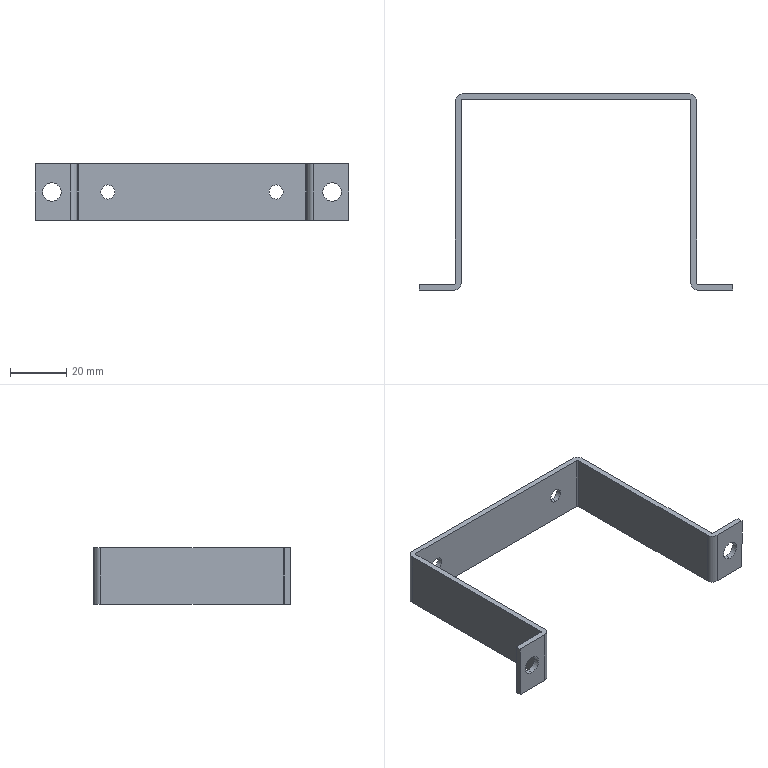Part | STEP file | Support sheet metal | 1 solid | 30 faces | box 112 x 70 x 20 mm | volume 9602 mm3 | cylinder 16 | plane 14 | commonest cylinder face diameters 5 x8 1 x4 6.6 x4
STEP:
#1=CARTESIAN_POINT('',(30.,-2.,-2.5));
#2=VERTEX_POINT('',#1);
#3=CARTESIAN_POINT('',(30.,-2.,2.5));
#4=VERTEX_POINT('',#3);
#5=CARTESIAN_POINT('',(30.,-2.,0.));
#6=DIRECTION('',(0.,1.,0.));
#7=DIRECTION('',(0.,0.,1.));
#8=AXIS2_PLACEMENT_3D('',#5,#6,#7);
#9=CIRCLE('',#8,2.5);
#10=EDGE_CURVE('',#2,#4,#9,.T.);
#11=ORIENTED_EDGE('',*,*,#10,.F.);
#12=CARTESIAN_POINT('',(30.,0.,-2.5));
#13=VERTEX_POINT('',#12);
#14=CARTESIAN_POINT('',(30.,0.,-2.5));
#15=DIRECTION('',(0.,1.,0.));
#16=VECTOR('',#15,1000.);
#17=LINE('',#14,#16);
#18=EDGE_CURVE('',#2,#13,#17,.T.);
#19=ORIENTED_EDGE('',*,*,#18,.T.);
#20=CARTESIAN_POINT('',(30.,0.,2.5));
#21=VERTEX_POINT('',#20);
#22=CARTESIAN_POINT('',(30.,0.,0.));
#23=DIRECTION('',(0.,-1.,0.));
#24=DIRECTION('',(0.,0.,1.));
#25=AXIS2_PLACEMENT_3D('',#22,#23,#24);
#26=CIRCLE('',#25,2.5);
#27=EDGE_CURVE('',#21,#13,#26,.T.);
#28=ORIENTED_EDGE('',*,*,#27,.F.);
#29=CARTESIAN_POINT('',(30.,0.,2.5));
#30=DIRECTION('',(0.,1.,0.));
#31=VECTOR('',#30,1000.);
#32=LINE('',#29,#31);
#33=EDGE_CURVE('',#4,#21,#32,.T.);
#34=ORIENTED_EDGE('',*,*,#33,.F.);
#35=EDGE_LOOP('',(#11,#19,#28,#34));
#36=FACE_OUTER_BOUND('',#35,.T.);
#37=CARTESIAN_POINT('',(30.,0.,0.));
#38=DIRECTION('',(0.,1.,0.));
#39=DIRECTION('',(0.,0.,1.));
#40=AXIS2_PLACEMENT_3D('',#37,#38,#39);
#41=CYLINDRICAL_SURFACE('',#40,2.5);
#42=ADVANCED_FACE('',(#36),#41,.F.);
#43=CARTESIAN_POINT('',(-30.,-2.,-2.5));
#44=VERTEX_POINT('',#43);
#45=CARTESIAN_POINT('',(-30.,-2.,2.5));
#46=VERTEX_POINT('',#45);
#47=CARTESIAN_POINT('',(-30.,-2.,0.));
#48=DIRECTION('',(0.,1.,0.));
#49=DIRECTION('',(0.,0.,1.));
#50=AXIS2_PLACEMENT_3D('',#47,#48,#49);
#51=CIRCLE('',#50,2.5);
#52=EDGE_CURVE('',#44,#46,#51,.T.);
#53=ORIENTED_EDGE('',*,*,#52,.F.);
#54=CARTESIAN_POINT('',(-30.,0.,-2.5));
#55=VERTEX_POINT('',#54);
#56=CARTESIAN_POINT('',(-30.,0.,-2.5));
#57=DIRECTION('',(0.,1.,0.));
#58=VECTOR('',#57,1000.);
#59=LINE('',#56,#58);
#60=EDGE_CURVE('',#44,#55,#59,.T.);
#61=ORIENTED_EDGE('',*,*,#60,.T.);
#62=CARTESIAN_POINT('',(-30.,0.,2.5));
#63=VERTEX_POINT('',#62);
#64=CARTESIAN_POINT('',(-30.,0.,0.));
#65=DIRECTION('',(0.,-1.,0.));
#66=DIRECTION('',(0.,0.,1.));
#67=AXIS2_PLACEMENT_3D('',#64,#65,#66);
#68=CIRCLE('',#67,2.5);
#69=EDGE_CURVE('',#63,#55,#68,.T.);
#70=ORIENTED_EDGE('',*,*,#69,.F.);
#71=CARTESIAN_POINT('',(-30.,0.,2.5));
#72=DIRECTION('',(0.,1.,0.));
#73=VECTOR('',#72,1000.);
#74=LINE('',#71,#73);
#75=EDGE_CURVE('',#46,#63,#74,.T.);
#76=ORIENTED_EDGE('',*,*,#75,.F.);
#77=EDGE_LOOP('',(#53,#61,#70,#76));
#78=FACE_OUTER_BOUND('',#77,.T.);
#79=CARTESIAN_POINT('',(-30.,0.,0.));
#80=DIRECTION('',(0.,1.,0.));
#81=DIRECTION('',(0.,0.,1.));
#82=AXIS2_PLACEMENT_3D('',#79,#80,#81);
#83=CYLINDRICAL_SURFACE('',#82,2.5);
#84=ADVANCED_FACE('',(#78),#83,.F.);
#85=CARTESIAN_POINT('',(50.,-70.,-3.3));
#86=VERTEX_POINT('',#85);
#87=CARTESIAN_POINT('',(50.,-70.,3.3));
#88=VERTEX_POINT('',#87);
#89=CARTESIAN_POINT('',(50.,-70.,0.));
#90=DIRECTION('',(0.,1.,0.));
#91=DIRECTION('',(0.,0.,1.));
#92=AXIS2_PLACEMENT_3D('',#89,#90,#91);
#93=CIRCLE('',#92,3.3);
#94=EDGE_CURVE('',#86,#88,#93,.T.);
#95=ORIENTED_EDGE('',*,*,#94,.F.);
#96=CARTESIAN_POINT('',(50.,-68.,-3.3));
#97=VERTEX_POINT('',#96);
#98=CARTESIAN_POINT('',(50.,-68.,-3.3));
#99=DIRECTION('',(0.,1.,0.));
#100=VECTOR('',#99,1000.);
#101=LINE('',#98,#100);
#102=EDGE_CURVE('',#86,#97,#101,.T.);
#103=ORIENTED_EDGE('',*,*,#102,.T.);
#104=CARTESIAN_POINT('',(50.,-68.,3.3));
#105=VERTEX_POINT('',#104);
#106=CARTESIAN_POINT('',(50.,-68.,0.));
#107=DIRECTION('',(0.,-1.,0.));
#108=DIRECTION('',(0.,0.,1.));
#109=AXIS2_PLACEMENT_3D('',#106,#107,#108);
#110=CIRCLE('',#109,3.3);
#111=EDGE_CURVE('',#105,#97,#110,.T.);
#112=ORIENTED_EDGE('',*,*,#111,.F.);
#113=CARTESIAN_POINT('',(50.,-68.,3.3));
#114=DIRECTION('',(0.,1.,0.));
#115=VECTOR('',#114,1000.);
#116=LINE('',#113,#115);
#117=EDGE_CURVE('',#88,#105,#116,.T.);
#118=ORIENTED_EDGE('',*,*,#117,.F.);
#119=EDGE_LOOP('',(#95,#103,#112,#118));
#120=FACE_OUTER_BOUND('',#119,.T.);
#121=CARTESIAN_POINT('',(50.,-68.,0.));
#122=DIRECTION('',(0.,1.,0.));
#123=DIRECTION('',(0.,0.,1.));
#124=AXIS2_PLACEMENT_3D('',#121,#122,#123);
#125=CYLINDRICAL_SURFACE('',#124,3.3);
#126=ADVANCED_FACE('',(#120),#125,.F.);
#127=CARTESIAN_POINT('',(-50.,-70.,-3.3));
#128=VERTEX_POINT('',#127);
#129=CARTESIAN_POINT('',(-50.,-70.,3.3));
#130=VERTEX_POINT('',#129);
#131=CARTESIAN_POINT('',(-50.,-70.,0.));
#132=DIRECTION('',(0.,1.,0.));
#133=DIRECTION('',(0.,0.,1.));
#134=AXIS2_PLACEMENT_3D('',#131,#132,#133);
#135=CIRCLE('',#134,3.3);
#136=EDGE_CURVE('',#128,#130,#135,.T.);
#137=ORIENTED_EDGE('',*,*,#136,.F.);
#138=CARTESIAN_POINT('',(-50.,-68.,-3.3));
#139=VERTEX_POINT('',#138);
#140=CARTESIAN_POINT('',(-50.,-68.,-3.3));
#141=DIRECTION('',(0.,1.,0.));
#142=VECTOR('',#141,1000.);
#143=LINE('',#140,#142);
#144=EDGE_CURVE('',#128,#139,#143,.T.);
#145=ORIENTED_EDGE('',*,*,#144,.T.);
#146=CARTESIAN_POINT('',(-50.,-68.,3.3));
#147=VERTEX_POINT('',#146);
#148=CARTESIAN_POINT('',(-50.,-68.,0.));
#149=DIRECTION('',(0.,-1.,0.));
#150=DIRECTION('',(0.,0.,1.));
#151=AXIS2_PLACEMENT_3D('',#148,#149,#150);
#152=CIRCLE('',#151,3.3);
#153=EDGE_CURVE('',#147,#139,#152,.T.);
#154=ORIENTED_EDGE('',*,*,#153,.F.);
#155=CARTESIAN_POINT('',(-50.,-68.,3.3));
#156=DIRECTION('',(0.,1.,0.));
#157=VECTOR('',#156,1000.);
#158=LINE('',#155,#157);
#159=EDGE_CURVE('',#130,#147,#158,.T.);
#160=ORIENTED_EDGE('',*,*,#159,.F.);
#161=EDGE_LOOP('',(#137,#145,#154,#160));
#162=FACE_OUTER_BOUND('',#161,.T.);
#163=CARTESIAN_POINT('',(-50.,-68.,0.));
#164=DIRECTION('',(0.,1.,0.));
#165=DIRECTION('',(0.,0.,1.));
#166=AXIS2_PLACEMENT_3D('',#163,#164,#165);
#167=CYLINDRICAL_SURFACE('',#166,3.3);
#168=ADVANCED_FACE('',(#162),#167,.F.);
#169=CARTESIAN_POINT('',(-40.5,0.,10.));
#170=VERTEX_POINT('',#169);
#171=CARTESIAN_POINT('',(40.5,0.,10.));
#172=VERTEX_POINT('',#171);
#173=CARTESIAN_POINT('',(-43.,0.,10.));
#174=DIRECTION('',(1.,0.,0.));
#175=VECTOR('',#174,1000.);
#176=LINE('',#173,#175);
#177=EDGE_CURVE('',#170,#172,#176,.T.);
#178=ORIENTED_EDGE('',*,*,#177,.T.);
#179=CARTESIAN_POINT('',(40.5,0.,-10.));
#180=VERTEX_POINT('',#179);
#181=CARTESIAN_POINT('',(40.5,0.,10.));
#182=DIRECTION('',(0.,0.,-1.));
#183=VECTOR('',#182,1000.);
#184=LINE('',#181,#183);
#185=EDGE_CURVE('',#172,#180,#184,.T.);
#186=ORIENTED_EDGE('',*,*,#185,.T.);
#187=CARTESIAN_POINT('',(-40.5,0.,-10.));
#188=VERTEX_POINT('',#187);
#189=CARTESIAN_POINT('',(-43.,0.,-10.));
#190=DIRECTION('',(-1.,0.,0.));
#191=VECTOR('',#190,1000.);
#192=LINE('',#189,#191);
#193=EDGE_CURVE('',#180,#188,#192,.T.);
#194=ORIENTED_EDGE('',*,*,#193,.T.);
#195=CARTESIAN_POINT('',(-40.5,0.,10.));
#196=DIRECTION('',(0.,0.,1.));
#197=VECTOR('',#196,1000.);
#198=LINE('',#195,#197);
#199=EDGE_CURVE('',#188,#170,#198,.T.);
#200=ORIENTED_EDGE('',*,*,#199,.T.);
#201=EDGE_LOOP('',(#178,#186,#194,#200));
#202=FACE_OUTER_BOUND('',#201,.T.);
#203=ORIENTED_EDGE('',*,*,#27,.T.);
#204=CARTESIAN_POINT('',(30.,0.,0.));
#205=DIRECTION('',(0.,-1.,0.));
#206=DIRECTION('',(0.,0.,1.));
#207=AXIS2_PLACEMENT_3D('',#204,#205,#206);
#208=CIRCLE('',#207,2.5);
#209=EDGE_CURVE('',#13,#21,#208,.T.);
#210=ORIENTED_EDGE('',*,*,#209,.T.);
#211=EDGE_LOOP('',(#203,#210));
#212=FACE_BOUND('',#211,.T.);
#213=ORIENTED_EDGE('',*,*,#69,.T.);
#214=CARTESIAN_POINT('',(-30.,0.,0.));
#215=DIRECTION('',(0.,-1.,0.));
#216=DIRECTION('',(0.,0.,1.));
#217=AXIS2_PLACEMENT_3D('',#214,#215,#216);
#218=CIRCLE('',#217,2.5);
#219=EDGE_CURVE('',#55,#63,#218,.T.);
#220=ORIENTED_EDGE('',*,*,#219,.T.);
#221=EDGE_LOOP('',(#213,#220));
#222=FACE_BOUND('',#221,.T.);
#223=CARTESIAN_POINT('',(-43.,0.,10.));
#224=DIRECTION('',(0.,1.,0.));
#225=DIRECTION('',(0.,0.,1.));
#226=AXIS2_PLACEMENT_3D('',#223,#224,#225);
#227=PLANE('',#226);
#228=ADVANCED_FACE('',(#202,#212,#222),#227,.T.);
#229=CARTESIAN_POINT('',(43.,-2.5,10.));
#230=VERTEX_POINT('',#229);
#231=CARTESIAN_POINT('',(40.5,-2.5,10.));
#232=DIRECTION('',(0.,0.,-1.));
#233=DIRECTION('',(-1.,0.,0.));
#234=AXIS2_PLACEMENT_3D('',#231,#232,#233);
#235=CIRCLE('',#234,2.5);
#236=EDGE_CURVE('',#172,#230,#235,.T.);
#237=ORIENTED_EDGE('',*,*,#236,.T.);
#238=CARTESIAN_POINT('',(43.,-2.5,-10.));
#239=VERTEX_POINT('',#238);
#240=CARTESIAN_POINT('',(43.,-2.5,10.));
#241=DIRECTION('',(0.,0.,-1.));
#242=VECTOR('',#241,1000.);
#243=LINE('',#240,#242);
#244=EDGE_CURVE('',#230,#239,#243,.T.);
#245=ORIENTED_EDGE('',*,*,#244,.T.);
#246=CARTESIAN_POINT('',(40.5,-2.5,-10.));
#247=DIRECTION('',(0.,0.,1.));
#248=DIRECTION('',(-1.,0.,0.));
#249=AXIS2_PLACEMENT_3D('',#246,#247,#248);
#250=CIRCLE('',#249,2.5);
#251=EDGE_CURVE('',#239,#180,#250,.T.);
#252=ORIENTED_EDGE('',*,*,#251,.T.);
#253=ORIENTED_EDGE('',*,*,#185,.F.);
#254=EDGE_LOOP('',(#237,#245,#252,#253));
#255=FACE_OUTER_BOUND('',#254,.T.);
#256=CARTESIAN_POINT('',(40.5,-2.5,10.));
#257=DIRECTION('',(0.,0.,-1.));
#258=DIRECTION('',(-1.,0.,0.));
#259=AXIS2_PLACEMENT_3D('',#256,#257,#258);
#260=CYLINDRICAL_SURFACE('',#259,2.5);
#261=ADVANCED_FACE('',(#255),#260,.T.);
#262=CARTESIAN_POINT('',(-40.5,-2.,10.));
#263=VERTEX_POINT('',#262);
#264=CARTESIAN_POINT('',(40.5,-2.,10.));
#265=VERTEX_POINT('',#264);
#266=CARTESIAN_POINT('',(-41.,-2.,10.));
#267=DIRECTION('',(1.,0.,0.));
#268=VECTOR('',#267,1000.);
#269=LINE('',#266,#268);
#270=EDGE_CURVE('',#263,#265,#269,.T.);
#271=ORIENTED_EDGE('',*,*,#270,.T.);
#272=CARTESIAN_POINT('',(41.,-2.5,10.));
#273=VERTEX_POINT('',#272);
#274=CARTESIAN_POINT('',(40.5,-2.5,10.));
#275=DIRECTION('',(0.,0.,-1.));
#276=DIRECTION('',(-1.,0.,0.));
#277=AXIS2_PLACEMENT_3D('',#274,#275,#276);
#278=CIRCLE('',#277,0.5);
#279=EDGE_CURVE('',#265,#273,#278,.T.);
#280=ORIENTED_EDGE('',*,*,#279,.T.);
#281=CARTESIAN_POINT('',(41.,-67.5,10.));
#282=VERTEX_POINT('',#281);
#283=CARTESIAN_POINT('',(41.,-2.,10.));
#284=DIRECTION('',(0.,-1.,0.));
#285=VECTOR('',#284,1000.);
#286=LINE('',#283,#285);
#287=EDGE_CURVE('',#273,#282,#286,.T.);
#288=ORIENTED_EDGE('',*,*,#287,.T.);
#289=CARTESIAN_POINT('',(43.5,-70.,10.));
#290=VERTEX_POINT('',#289);
#291=CARTESIAN_POINT('',(43.5,-67.5,10.));
#292=DIRECTION('',(0.,0.,1.));
#293=DIRECTION('',(-1.,0.,0.));
#294=AXIS2_PLACEMENT_3D('',#291,#292,#293);
#295=CIRCLE('',#294,2.5);
#296=EDGE_CURVE('',#282,#290,#295,.T.);
#297=ORIENTED_EDGE('',*,*,#296,.T.);
#298=CARTESIAN_POINT('',(56.,-70.,10.));
#299=VERTEX_POINT('',#298);
#300=CARTESIAN_POINT('',(43.,-70.,10.));
#301=DIRECTION('',(-1.,0.,0.));
#302=VECTOR('',#301,1000.);
#303=LINE('',#300,#302);
#304=EDGE_CURVE('',#299,#290,#303,.T.);
#305=ORIENTED_EDGE('',*,*,#304,.F.);
#306=CARTESIAN_POINT('',(56.,-68.,10.));
#307=VERTEX_POINT('',#306);
#308=CARTESIAN_POINT('',(56.,-70.,10.));
#309=DIRECTION('',(0.,1.,0.));
#310=VECTOR('',#309,1000.);
#311=LINE('',#308,#310);
#312=EDGE_CURVE('',#299,#307,#311,.T.);
#313=ORIENTED_EDGE('',*,*,#312,.T.);
#314=CARTESIAN_POINT('',(43.5,-68.,10.));
#315=VERTEX_POINT('',#314);
#316=CARTESIAN_POINT('',(0.,-68.,10.));
#317=DIRECTION('',(1.,0.,0.));
#318=VECTOR('',#317,1000.);
#319=LINE('',#316,#318);
#320=EDGE_CURVE('',#315,#307,#319,.T.);
#321=ORIENTED_EDGE('',*,*,#320,.F.);
#322=CARTESIAN_POINT('',(43.,-67.5,10.));
#323=VERTEX_POINT('',#322);
#324=CARTESIAN_POINT('',(43.5,-67.5,10.));
#325=DIRECTION('',(0.,0.,-1.));
#326=DIRECTION('',(-1.,0.,0.));
#327=AXIS2_PLACEMENT_3D('',#324,#325,#326);
#328=CIRCLE('',#327,0.5);
#329=EDGE_CURVE('',#315,#323,#328,.T.);
#330=ORIENTED_EDGE('',*,*,#329,.T.);
#331=CARTESIAN_POINT('',(43.,0.,10.));
#332=DIRECTION('',(0.,-1.,0.));
#333=VECTOR('',#332,1000.);
#334=LINE('',#331,#333);
#335=EDGE_CURVE('',#230,#323,#334,.T.);
#336=ORIENTED_EDGE('',*,*,#335,.F.);
#337=ORIENTED_EDGE('',*,*,#236,.F.);
#338=ORIENTED_EDGE('',*,*,#177,.F.);
#339=CARTESIAN_POINT('',(-43.,-2.5,10.));
#340=VERTEX_POINT('',#339);
#341=CARTESIAN_POINT('',(-40.5,-2.5,10.));
#342=DIRECTION('',(0.,0.,-1.));
#343=DIRECTION('',(-1.,0.,0.));
#344=AXIS2_PLACEMENT_3D('',#341,#342,#343);
#345=CIRCLE('',#344,2.5);
#346=EDGE_CURVE('',#340,#170,#345,.T.);
#347=ORIENTED_EDGE('',*,*,#346,.F.);
#348=CARTESIAN_POINT('',(-43.,-67.5,10.));
#349=VERTEX_POINT('',#348);
#350=CARTESIAN_POINT('',(-43.,-70.,10.));
#351=DIRECTION('',(0.,1.,0.));
#352=VECTOR('',#351,1000.);
#353=LINE('',#350,#352);
#354=EDGE_CURVE('',#349,#340,#353,.T.);
#355=ORIENTED_EDGE('',*,*,#354,.F.);
#356=CARTESIAN_POINT('',(-43.5,-68.,10.));
#357=VERTEX_POINT('',#356);
#358=CARTESIAN_POINT('',(-43.5,-67.5,10.));
#359=DIRECTION('',(0.,0.,-1.));
#360=DIRECTION('',(1.,0.,0.));
#361=AXIS2_PLACEMENT_3D('',#358,#359,#360);
#362=CIRCLE('',#361,0.5);
#363=EDGE_CURVE('',#349,#357,#362,.T.);
#364=ORIENTED_EDGE('',*,*,#363,.T.);
#365=CARTESIAN_POINT('',(-56.,-68.,10.));
#366=VERTEX_POINT('',#365);
#367=CARTESIAN_POINT('',(0.,-68.,10.));
#368=DIRECTION('',(1.,0.,0.));
#369=VECTOR('',#368,1000.);
#370=LINE('',#367,#369);
#371=EDGE_CURVE('',#366,#357,#370,.T.);
#372=ORIENTED_EDGE('',*,*,#371,.F.);
#373=CARTESIAN_POINT('',(-56.,-70.,10.));
#374=VERTEX_POINT('',#373);
#375=CARTESIAN_POINT('',(-56.,-70.,10.));
#376=DIRECTION('',(0.,1.,0.));
#377=VECTOR('',#376,1000.);
#378=LINE('',#375,#377);
#379=EDGE_CURVE('',#374,#366,#378,.T.);
#380=ORIENTED_EDGE('',*,*,#379,.F.);
#381=CARTESIAN_POINT('',(-43.5,-70.,10.));
#382=VERTEX_POINT('',#381);
#383=CARTESIAN_POINT('',(-56.,-70.,10.));
#384=DIRECTION('',(-1.,0.,0.));
#385=VECTOR('',#384,1000.);
#386=LINE('',#383,#385);
#387=EDGE_CURVE('',#382,#374,#386,.T.);
#388=ORIENTED_EDGE('',*,*,#387,.F.);
#389=CARTESIAN_POINT('',(-41.,-67.5,10.));
#390=VERTEX_POINT('',#389);
#391=CARTESIAN_POINT('',(-43.5,-67.5,10.));
#392=DIRECTION('',(0.,0.,-1.));
#393=DIRECTION('',(1.,0.,0.));
#394=AXIS2_PLACEMENT_3D('',#391,#392,#393);
#395=CIRCLE('',#394,2.5);
#396=EDGE_CURVE('',#390,#382,#395,.T.);
#397=ORIENTED_EDGE('',*,*,#396,.F.);
#398=CARTESIAN_POINT('',(-41.,-2.5,10.));
#399=VERTEX_POINT('',#398);
#400=CARTESIAN_POINT('',(-41.,-2.5,10.));
#401=DIRECTION('',(0.,1.,0.));
#402=VECTOR('',#401,1000.);
#403=LINE('',#400,#402);
#404=EDGE_CURVE('',#390,#399,#403,.T.);
#405=ORIENTED_EDGE('',*,*,#404,.T.);
#406=CARTESIAN_POINT('',(-40.5,-2.5,10.));
#407=DIRECTION('',(0.,0.,-1.));
#408=DIRECTION('',(-1.,0.,0.));
#409=AXIS2_PLACEMENT_3D('',#406,#407,#408);
#410=CIRCLE('',#409,0.5);
#411=EDGE_CURVE('',#399,#263,#410,.T.);
#412=ORIENTED_EDGE('',*,*,#411,.T.);
#413=EDGE_LOOP('',(#271,#280,#288,#297,#305,#313,#321,#330,#336,#337,#338,#347,#355,#364,#372,#380,#388,#397,#405,#412));
#414=FACE_OUTER_BOUND('',#413,.T.);
#415=CARTESIAN_POINT('',(-41.,-2.5,10.));
#416=DIRECTION('',(0.,0.,1.));
#417=DIRECTION('',(1.,0.,0.));
#418=AXIS2_PLACEMENT_3D('',#415,#416,#417);
#419=PLANE('',#418);
#420=ADVANCED_FACE('',(#414),#419,.T.);
#421=ORIENTED_EDGE('',*,*,#346,.T.);
#422=ORIENTED_EDGE('',*,*,#199,.F.);
#423=CARTESIAN_POINT('',(-43.,-2.5,-10.));
#424=VERTEX_POINT('',#423);
#425=CARTESIAN_POINT('',(-40.5,-2.5,-10.));
#426=DIRECTION('',(0.,0.,1.));
#427=DIRECTION('',(-1.,0.,0.));
#428=AXIS2_PLACEMENT_3D('',#425,#426,#427);
#429=CIRCLE('',#428,2.5);
#430=EDGE_CURVE('',#188,#424,#429,.T.);
#431=ORIENTED_EDGE('',*,*,#430,.T.);
#432=CARTESIAN_POINT('',(-43.,-2.5,10.));
#433=DIRECTION('',(0.,0.,1.));
#434=VECTOR('',#433,1000.);
#435=LINE('',#432,#434);
#436=EDGE_CURVE('',#424,#340,#435,.T.);
#437=ORIENTED_EDGE('',*,*,#436,.T.);
#438=EDGE_LOOP('',(#421,#422,#431,#437));
#439=FACE_OUTER_BOUND('',#438,.T.);
#440=CARTESIAN_POINT('',(-40.5,-2.5,10.));
#441=DIRECTION('',(0.,0.,-1.));
#442=DIRECTION('',(-1.,0.,0.));
#443=AXIS2_PLACEMENT_3D('',#440,#441,#442);
#444=CYLINDRICAL_SURFACE('',#443,2.5);
#445=ADVANCED_FACE('',(#439),#444,.T.);
#446=CARTESIAN_POINT('',(40.5,-2.,-10.));
#447=VERTEX_POINT('',#446);
#448=CARTESIAN_POINT('',(-40.5,-2.,-10.));
#449=VERTEX_POINT('',#448);
#450=CARTESIAN_POINT('',(41.,-2.,-10.));
#451=DIRECTION('',(-1.,0.,0.));
#452=VECTOR('',#451,1000.);
#453=LINE('',#450,#452);
#454=EDGE_CURVE('',#447,#449,#453,.T.);
#455=ORIENTED_EDGE('',*,*,#454,.T.);
#456=CARTESIAN_POINT('',(-41.,-2.5,-10.));
#457=VERTEX_POINT('',#456);
#458=CARTESIAN_POINT('',(-40.5,-2.5,-10.));
#459=DIRECTION('',(0.,0.,1.));
#460=DIRECTION('',(-1.,0.,0.));
#461=AXIS2_PLACEMENT_3D('',#458,#459,#460);
#462=CIRCLE('',#461,0.5);
#463=EDGE_CURVE('',#449,#457,#462,.T.);
#464=ORIENTED_EDGE('',*,*,#463,.T.);
#465=CARTESIAN_POINT('',(-41.,-67.5,-10.));
#466=VERTEX_POINT('',#465);
#467=CARTESIAN_POINT('',(-41.,-2.,-10.));
#468=DIRECTION('',(0.,-1.,0.));
#469=VECTOR('',#468,1000.);
#470=LINE('',#467,#469);
#471=EDGE_CURVE('',#457,#466,#470,.T.);
#472=ORIENTED_EDGE('',*,*,#471,.T.);
#473=CARTESIAN_POINT('',(-43.5,-70.,-10.));
#474=VERTEX_POINT('',#473);
#475=CARTESIAN_POINT('',(-43.5,-67.5,-10.));
#476=DIRECTION('',(0.,0.,-1.));
#477=DIRECTION('',(1.,0.,0.));
#478=AXIS2_PLACEMENT_3D('',#475,#476,#477);
#479=CIRCLE('',#478,2.5);
#480=EDGE_CURVE('',#466,#474,#479,.T.);
#481=ORIENTED_EDGE('',*,*,#480,.T.);
#482=CARTESIAN_POINT('',(-56.,-70.,-10.));
#483=VERTEX_POINT('',#482);
#484=CARTESIAN_POINT('',(-43.,-70.,-10.));
#485=DIRECTION('',(1.,0.,0.));
#486=VECTOR('',#485,1000.);
#487=LINE('',#484,#486);
#488=EDGE_CURVE('',#483,#474,#487,.T.);
#489=ORIENTED_EDGE('',*,*,#488,.F.);
#490=CARTESIAN_POINT('',(-56.,-68.,-10.));
#491=VERTEX_POINT('',#490);
#492=CARTESIAN_POINT('',(-56.,-70.,-10.));
#493=DIRECTION('',(0.,1.,0.));
#494=VECTOR('',#493,1000.);
#495=LINE('',#492,#494);
#496=EDGE_CURVE('',#483,#491,#495,.T.);
#497=ORIENTED_EDGE('',*,*,#496,.T.);
#498=CARTESIAN_POINT('',(-43.5,-68.,-10.));
#499=VERTEX_POINT('',#498);
#500=CARTESIAN_POINT('',(0.,-68.,-10.));
#501=DIRECTION('',(-1.,0.,0.));
#502=VECTOR('',#501,1000.);
#503=LINE('',#500,#502);
#504=EDGE_CURVE('',#499,#491,#503,.T.);
#505=ORIENTED_EDGE('',*,*,#504,.F.);
#506=CARTESIAN_POINT('',(-43.,-67.5,-10.));
#507=VERTEX_POINT('',#506);
#508=CARTESIAN_POINT('',(-43.5,-67.5,-10.));
#509=DIRECTION('',(0.,0.,1.));
#510=DIRECTION('',(1.,0.,0.));
#511=AXIS2_PLACEMENT_3D('',#508,#509,#510);
#512=CIRCLE('',#511,0.5);
#513=EDGE_CURVE('',#499,#507,#512,.T.);
#514=ORIENTED_EDGE('',*,*,#513,.T.);
#515=CARTESIAN_POINT('',(-43.,-70.,-10.));
#516=DIRECTION('',(0.,-1.,0.));
#517=VECTOR('',#516,1000.);
#518=LINE('',#515,#517);
#519=EDGE_CURVE('',#424,#507,#518,.T.);
#520=ORIENTED_EDGE('',*,*,#519,.F.);
#521=ORIENTED_EDGE('',*,*,#430,.F.);
#522=ORIENTED_EDGE('',*,*,#193,.F.);
#523=ORIENTED_EDGE('',*,*,#251,.F.);
#524=CARTESIAN_POINT('',(43.,-67.5,-10.));
#525=VERTEX_POINT('',#524);
#526=CARTESIAN_POINT('',(43.,0.,-10.));
#527=DIRECTION('',(0.,1.,0.));
#528=VECTOR('',#527,1000.);
#529=LINE('',#526,#528);
#530=EDGE_CURVE('',#525,#239,#529,.T.);
#531=ORIENTED_EDGE('',*,*,#530,.F.);
#532=CARTESIAN_POINT('',(43.5,-68.,-10.));
#533=VERTEX_POINT('',#532);
#534=CARTESIAN_POINT('',(43.5,-67.5,-10.));
#535=DIRECTION('',(0.,0.,1.));
#536=DIRECTION('',(-1.,0.,0.));
#537=AXIS2_PLACEMENT_3D('',#534,#535,#536);
#538=CIRCLE('',#537,0.5);
#539=EDGE_CURVE('',#525,#533,#538,.T.);
#540=ORIENTED_EDGE('',*,*,#539,.T.);
#541=CARTESIAN_POINT('',(56.,-68.,-10.));
#542=VERTEX_POINT('',#541);
#543=CARTESIAN_POINT('',(0.,-68.,-10.));
#544=DIRECTION('',(-1.,0.,0.));
#545=VECTOR('',#544,1000.);
#546=LINE('',#543,#545);
#547=EDGE_CURVE('',#542,#533,#546,.T.);
#548=ORIENTED_EDGE('',*,*,#547,.F.);
#549=CARTESIAN_POINT('',(56.,-70.,-10.));
#550=VERTEX_POINT('',#549);
#551=CARTESIAN_POINT('',(56.,-70.,-10.));
#552=DIRECTION('',(0.,1.,0.));
#553=VECTOR('',#552,1000.);
#554=LINE('',#551,#553);
#555=EDGE_CURVE('',#550,#542,#554,.T.);
#556=ORIENTED_EDGE('',*,*,#555,.F.);
#557=CARTESIAN_POINT('',(43.5,-70.,-10.));
#558=VERTEX_POINT('',#557);
#559=CARTESIAN_POINT('',(56.,-70.,-10.));
#560=DIRECTION('',(1.,0.,0.));
#561=VECTOR('',#560,1000.);
#562=LINE('',#559,#561);
#563=EDGE_CURVE('',#558,#550,#562,.T.);
#564=ORIENTED_EDGE('',*,*,#563,.F.);
#565=CARTESIAN_POINT('',(41.,-67.5,-10.));
#566=VERTEX_POINT('',#565);
#567=CARTESIAN_POINT('',(43.5,-67.5,-10.));
#568=DIRECTION('',(0.,0.,1.));
#569=DIRECTION('',(-1.,0.,0.));
#570=AXIS2_PLACEMENT_3D('',#567,#568,#569);
#571=CIRCLE('',#570,2.5);
#572=EDGE_CURVE('',#566,#558,#571,.T.);
#573=ORIENTED_EDGE('',*,*,#572,.F.);
#574=CARTESIAN_POINT('',(41.,-2.5,-10.));
#575=VERTEX_POINT('',#574);
#576=CARTESIAN_POINT('',(41.,-2.5,-10.));
#577=DIRECTION('',(0.,-1.,0.));
#578=VECTOR('',#577,1000.);
#579=LINE('',#576,#578);
#580=EDGE_CURVE('',#575,#566,#579,.T.);
#581=ORIENTED_EDGE('',*,*,#580,.F.);
#582=CARTESIAN_POINT('',(40.5,-2.5,-10.));
#583=DIRECTION('',(0.,0.,1.));
#584=DIRECTION('',(-1.,0.,0.));
#585=AXIS2_PLACEMENT_3D('',#582,#583,#584);
#586=CIRCLE('',#585,0.5);
#587=EDGE_CURVE('',#575,#447,#586,.T.);
#588=ORIENTED_EDGE('',*,*,#587,.T.);
#589=EDGE_LOOP('',(#455,#464,#472,#481,#489,#497,#505,#514,#520,#521,#522,#523,#531,#540,#548,#556,#564,#573,#581,#588));
#590=FACE_OUTER_BOUND('',#589,.T.);
#591=CARTESIAN_POINT('',(41.,-2.5,-10.));
#592=DIRECTION('',(0.,0.,-1.));
#593=DIRECTION('',(-1.,0.,0.));
#594=AXIS2_PLACEMENT_3D('',#591,#592,#593);
#595=PLANE('',#594);
#596=ADVANCED_FACE('',(#590),#595,.T.);
#597=ORIENTED_EDGE('',*,*,#18,.F.);
#598=CARTESIAN_POINT('',(30.,-2.,0.));
#599=DIRECTION('',(0.,1.,0.));
#600=DIRECTION('',(0.,0.,1.));
#601=AXIS2_PLACEMENT_3D('',#598,#599,#600);
#602=CIRCLE('',#601,2.5);
#603=EDGE_CURVE('',#4,#2,#602,.T.);
#604=ORIENTED_EDGE('',*,*,#603,.F.);
#605=ORIENTED_EDGE('',*,*,#33,.T.);
#606=ORIENTED_EDGE('',*,*,#209,.F.);
#607=EDGE_LOOP('',(#597,#604,#605,#606));
#608=FACE_OUTER_BOUND('',#607,.T.);
#609=CARTESIAN_POINT('',(30.,0.,0.));
#610=DIRECTION('',(0.,1.,0.));
#611=DIRECTION('',(0.,0.,1.));
#612=AXIS2_PLACEMENT_3D('',#609,#610,#611);
#613=CYLINDRICAL_SURFACE('',#612,2.5);
#614=ADVANCED_FACE('',(#608),#613,.F.);
#615=ORIENTED_EDGE('',*,*,#60,.F.);
#616=CARTESIAN_POINT('',(-30.,-2.,0.));
#617=DIRECTION('',(0.,1.,0.));
#618=DIRECTION('',(0.,0.,1.));
#619=AXIS2_PLACEMENT_3D('',#616,#617,#618);
#620=CIRCLE('',#619,2.5);
#621=EDGE_CURVE('',#46,#44,#620,.T.);
#622=ORIENTED_EDGE('',*,*,#621,.F.);
#623=ORIENTED_EDGE('',*,*,#75,.T.);
#624=ORIENTED_EDGE('',*,*,#219,.F.);
#625=EDGE_LOOP('',(#615,#622,#623,#624));
#626=FACE_OUTER_BOUND('',#625,.T.);
#627=CARTESIAN_POINT('',(-30.,0.,0.));
#628=DIRECTION('',(0.,1.,0.));
#629=DIRECTION('',(0.,0.,1.));
#630=AXIS2_PLACEMENT_3D('',#627,#628,#629);
#631=CYLINDRICAL_SURFACE('',#630,2.5);
#632=ADVANCED_FACE('',(#626),#631,.F.);
#633=ORIENTED_EDGE('',*,*,#530,.T.);
#634=ORIENTED_EDGE('',*,*,#244,.F.);
#635=ORIENTED_EDGE('',*,*,#335,.T.);
#636=CARTESIAN_POINT('',(43.,-67.5,10.));
#637=DIRECTION('',(0.,0.,-1.));
#638=VECTOR('',#637,1000.);
#639=LINE('',#636,#638);
#640=EDGE_CURVE('',#323,#525,#639,.T.);
#641=ORIENTED_EDGE('',*,*,#640,.T.);
#642=EDGE_LOOP('',(#633,#634,#635,#641));
#643=FACE_OUTER_BOUND('',#642,.T.);
#644=CARTESIAN_POINT('',(43.,0.,10.));
#645=DIRECTION('',(1.,0.,0.));
#646=DIRECTION('',(0.,1.,0.));
#647=AXIS2_PLACEMENT_3D('',#644,#645,#646);
#648=PLANE('',#647);
#649=ADVANCED_FACE('',(#643),#648,.T.);
#650=CARTESIAN_POINT('',(40.5,-2.,10.));
#651=DIRECTION('',(0.,0.,-1.));
#652=VECTOR('',#651,1000.);
#653=LINE('',#650,#652);
#654=EDGE_CURVE('',#265,#447,#653,.T.);
#655=ORIENTED_EDGE('',*,*,#654,.F.);
#656=ORIENTED_EDGE('',*,*,#270,.F.);
#657=CARTESIAN_POINT('',(-40.5,-2.,10.));
#658=DIRECTION('',(0.,0.,1.));
#659=VECTOR('',#658,1000.);
#660=LINE('',#657,#659);
#661=EDGE_CURVE('',#449,#263,#660,.T.);
#662=ORIENTED_EDGE('',*,*,#661,.F.);
#663=ORIENTED_EDGE('',*,*,#454,.F.);
#664=EDGE_LOOP('',(#655,#656,#662,#663));
#665=FACE_OUTER_BOUND('',#664,.T.);
#666=ORIENTED_EDGE('',*,*,#603,.T.);
#667=ORIENTED_EDGE('',*,*,#10,.T.);
#668=EDGE_LOOP('',(#666,#667));
#669=FACE_BOUND('',#668,.T.);
#670=ORIENTED_EDGE('',*,*,#621,.T.);
#671=ORIENTED_EDGE('',*,*,#52,.T.);
#672=EDGE_LOOP('',(#670,#671));
#673=FACE_BOUND('',#672,.T.);
#674=CARTESIAN_POINT('',(-43.,-2.,10.));
#675=DIRECTION('',(0.,1.,0.));
#676=DIRECTION('',(0.,0.,1.));
#677=AXIS2_PLACEMENT_3D('',#674,#675,#676);
#678=PLANE('',#677);
#679=ADVANCED_FACE('',(#665,#669,#673),#678,.F.);
#680=ORIENTED_EDGE('',*,*,#354,.T.);
#681=ORIENTED_EDGE('',*,*,#436,.F.);
#682=ORIENTED_EDGE('',*,*,#519,.T.);
#683=CARTESIAN_POINT('',(-43.,-67.5,10.));
#684=DIRECTION('',(0.,0.,1.));
#685=VECTOR('',#684,1000.);
#686=LINE('',#683,#685);
#687=EDGE_CURVE('',#507,#349,#686,.T.);
#688=ORIENTED_EDGE('',*,*,#687,.T.);
#689=EDGE_LOOP('',(#680,#681,#682,#688));
#690=FACE_OUTER_BOUND('',#689,.T.);
#691=CARTESIAN_POINT('',(-43.,-70.,10.));
#692=DIRECTION('',(-1.,0.,0.));
#693=DIRECTION('',(0.,-1.,0.));
#694=AXIS2_PLACEMENT_3D('',#691,#692,#693);
#695=PLANE('',#694);
#696=ADVANCED_FACE('',(#690),#695,.T.);
#697=ORIENTED_EDGE('',*,*,#329,.F.);
#698=CARTESIAN_POINT('',(43.5,-68.,-10.));
#699=DIRECTION('',(0.,0.,1.));
#700=VECTOR('',#699,1000.);
#701=LINE('',#698,#700);
#702=EDGE_CURVE('',#533,#315,#701,.T.);
#703=ORIENTED_EDGE('',*,*,#702,.F.);
#704=ORIENTED_EDGE('',*,*,#539,.F.);
#705=ORIENTED_EDGE('',*,*,#640,.F.);
#706=EDGE_LOOP('',(#697,#703,#704,#705));
#707=FACE_OUTER_BOUND('',#706,.T.);
#708=CARTESIAN_POINT('',(43.5,-67.5,-10.));
#709=DIRECTION('',(0.,0.,-1.));
#710=DIRECTION('',(-1.,0.,0.));
#711=AXIS2_PLACEMENT_3D('',#708,#709,#710);
#712=CYLINDRICAL_SURFACE('',#711,0.5);
#713=ADVANCED_FACE('',(#707),#712,.F.);
#714=CARTESIAN_POINT('',(41.,-2.5,10.));
#715=DIRECTION('',(0.,0.,-1.));
#716=VECTOR('',#715,1000.);
#717=LINE('',#714,#716);
#718=EDGE_CURVE('',#273,#575,#717,.T.);
#719=ORIENTED_EDGE('',*,*,#718,.F.);
#720=ORIENTED_EDGE('',*,*,#279,.F.);
#721=ORIENTED_EDGE('',*,*,#654,.T.);
#722=ORIENTED_EDGE('',*,*,#587,.F.);
#723=EDGE_LOOP('',(#719,#720,#721,#722));
#724=FACE_OUTER_BOUND('',#723,.T.);
#725=CARTESIAN_POINT('',(40.5,-2.5,10.));
#726=DIRECTION('',(0.,0.,-1.));
#727=DIRECTION('',(-1.,0.,0.));
#728=AXIS2_PLACEMENT_3D('',#725,#726,#727);
#729=CYLINDRICAL_SURFACE('',#728,0.5);
#730=ADVANCED_FACE('',(#724),#729,.F.);
#731=ORIENTED_EDGE('',*,*,#661,.T.);
#732=ORIENTED_EDGE('',*,*,#411,.F.);
#733=CARTESIAN_POINT('',(-41.,-2.5,10.));
#734=DIRECTION('',(0.,0.,1.));
#735=VECTOR('',#734,1000.);
#736=LINE('',#733,#735);
#737=EDGE_CURVE('',#457,#399,#736,.T.);
#738=ORIENTED_EDGE('',*,*,#737,.F.);
#739=ORIENTED_EDGE('',*,*,#463,.F.);
#740=EDGE_LOOP('',(#731,#732,#738,#739));
#741=FACE_OUTER_BOUND('',#740,.T.);
#742=CARTESIAN_POINT('',(-40.5,-2.5,10.));
#743=DIRECTION('',(0.,0.,-1.));
#744=DIRECTION('',(-1.,0.,0.));
#745=AXIS2_PLACEMENT_3D('',#742,#743,#744);
#746=CYLINDRICAL_SURFACE('',#745,0.5);
#747=ADVANCED_FACE('',(#741),#746,.F.);
#748=ORIENTED_EDGE('',*,*,#513,.F.);
#749=CARTESIAN_POINT('',(-43.5,-68.,10.));
#750=DIRECTION('',(0.,0.,-1.));
#751=VECTOR('',#750,1000.);
#752=LINE('',#749,#751);
#753=EDGE_CURVE('',#357,#499,#752,.T.);
#754=ORIENTED_EDGE('',*,*,#753,.F.);
#755=ORIENTED_EDGE('',*,*,#363,.F.);
#756=ORIENTED_EDGE('',*,*,#687,.F.);
#757=EDGE_LOOP('',(#748,#754,#755,#756));
#758=FACE_OUTER_BOUND('',#757,.T.);
#759=CARTESIAN_POINT('',(-43.5,-67.5,10.));
#760=DIRECTION('',(0.,0.,1.));
#761=DIRECTION('',(1.,0.,0.));
#762=AXIS2_PLACEMENT_3D('',#759,#760,#761);
#763=CYLINDRICAL_SURFACE('',#762,0.5);
#764=ADVANCED_FACE('',(#758),#763,.F.);
#765=ORIENTED_EDGE('',*,*,#287,.F.);
#766=ORIENTED_EDGE('',*,*,#718,.T.);
#767=ORIENTED_EDGE('',*,*,#580,.T.);
#768=CARTESIAN_POINT('',(41.,-67.5,10.));
#769=DIRECTION('',(0.,0.,-1.));
#770=VECTOR('',#769,1000.);
#771=LINE('',#768,#770);
#772=EDGE_CURVE('',#282,#566,#771,.T.);
#773=ORIENTED_EDGE('',*,*,#772,.F.);
#774=EDGE_LOOP('',(#765,#766,#767,#773));
#775=FACE_OUTER_BOUND('',#774,.T.);
#776=CARTESIAN_POINT('',(41.,0.,10.));
#777=DIRECTION('',(1.,0.,0.));
#778=DIRECTION('',(0.,1.,0.));
#779=AXIS2_PLACEMENT_3D('',#776,#777,#778);
#780=PLANE('',#779);
#781=ADVANCED_FACE('',(#775),#780,.F.);
#782=ORIENTED_EDGE('',*,*,#320,.T.);
#783=CARTESIAN_POINT('',(56.,-68.,0.));
#784=DIRECTION('',(0.,0.,-1.));
#785=VECTOR('',#784,1000.);
#786=LINE('',#783,#785);
#787=EDGE_CURVE('',#307,#542,#786,.T.);
#788=ORIENTED_EDGE('',*,*,#787,.T.);
#789=ORIENTED_EDGE('',*,*,#547,.T.);
#790=ORIENTED_EDGE('',*,*,#702,.T.);
#791=EDGE_LOOP('',(#782,#788,#789,#790));
#792=FACE_OUTER_BOUND('',#791,.T.);
#793=ORIENTED_EDGE('',*,*,#111,.T.);
#794=CARTESIAN_POINT('',(50.,-68.,0.));
#795=DIRECTION('',(0.,-1.,0.));
#796=DIRECTION('',(0.,0.,1.));
#797=AXIS2_PLACEMENT_3D('',#794,#795,#796);
#798=CIRCLE('',#797,3.3);
#799=EDGE_CURVE('',#97,#105,#798,.T.);
#800=ORIENTED_EDGE('',*,*,#799,.T.);
#801=EDGE_LOOP('',(#793,#800));
#802=FACE_BOUND('',#801,.T.);
#803=CARTESIAN_POINT('',(0.,-68.,0.));
#804=DIRECTION('',(0.,1.,0.));
#805=DIRECTION('',(-1.,0.,0.));
#806=AXIS2_PLACEMENT_3D('',#803,#804,#805);
#807=PLANE('',#806);
#808=ADVANCED_FACE('',(#792,#802),#807,.T.);
#809=ORIENTED_EDGE('',*,*,#471,.F.);
#810=ORIENTED_EDGE('',*,*,#737,.T.);
#811=ORIENTED_EDGE('',*,*,#404,.F.);
#812=CARTESIAN_POINT('',(-41.,-67.5,10.));
#813=DIRECTION('',(0.,0.,1.));
#814=VECTOR('',#813,1000.);
#815=LINE('',#812,#814);
#816=EDGE_CURVE('',#466,#390,#815,.T.);
#817=ORIENTED_EDGE('',*,*,#816,.F.);
#818=EDGE_LOOP('',(#809,#810,#811,#817));
#819=FACE_OUTER_BOUND('',#818,.T.);
#820=CARTESIAN_POINT('',(-41.,-70.,10.));
#821=DIRECTION('',(-1.,0.,0.));
#822=DIRECTION('',(0.,-1.,0.));
#823=AXIS2_PLACEMENT_3D('',#820,#821,#822);
#824=PLANE('',#823);
#825=ADVANCED_FACE('',(#819),#824,.F.);
#826=ORIENTED_EDGE('',*,*,#504,.T.);
#827=CARTESIAN_POINT('',(-56.,-68.,0.));
#828=DIRECTION('',(0.,0.,1.));
#829=VECTOR('',#828,1000.);
#830=LINE('',#827,#829);
#831=EDGE_CURVE('',#491,#366,#830,.T.);
#832=ORIENTED_EDGE('',*,*,#831,.T.);
#833=ORIENTED_EDGE('',*,*,#371,.T.);
#834=ORIENTED_EDGE('',*,*,#753,.T.);
#835=EDGE_LOOP('',(#826,#832,#833,#834));
#836=FACE_OUTER_BOUND('',#835,.T.);
#837=ORIENTED_EDGE('',*,*,#153,.T.);
#838=CARTESIAN_POINT('',(-50.,-68.,0.));
#839=DIRECTION('',(0.,-1.,0.));
#840=DIRECTION('',(0.,0.,1.));
#841=AXIS2_PLACEMENT_3D('',#838,#839,#840);
#842=CIRCLE('',#841,3.3);
#843=EDGE_CURVE('',#139,#147,#842,.T.);
#844=ORIENTED_EDGE('',*,*,#843,.T.);
#845=EDGE_LOOP('',(#837,#844));
#846=FACE_BOUND('',#845,.T.);
#847=CARTESIAN_POINT('',(0.,-68.,0.));
#848=DIRECTION('',(0.,1.,0.));
#849=DIRECTION('',(-1.,0.,0.));
#850=AXIS2_PLACEMENT_3D('',#847,#848,#849);
#851=PLANE('',#850);
#852=ADVANCED_FACE('',(#836,#846),#851,.T.);
#853=CARTESIAN_POINT('',(43.5,-70.,-10.));
#854=DIRECTION('',(0.,0.,1.));
#855=VECTOR('',#854,1000.);
#856=LINE('',#853,#855);
#857=EDGE_CURVE('',#558,#290,#856,.T.);
#858=ORIENTED_EDGE('',*,*,#857,.T.);
#859=ORIENTED_EDGE('',*,*,#296,.F.);
#860=ORIENTED_EDGE('',*,*,#772,.T.);
#861=ORIENTED_EDGE('',*,*,#572,.T.);
#862=EDGE_LOOP('',(#858,#859,#860,#861));
#863=FACE_OUTER_BOUND('',#862,.T.);
#864=CARTESIAN_POINT('',(43.5,-67.5,-10.));
#865=DIRECTION('',(0.,0.,-1.));
#866=DIRECTION('',(-1.,0.,0.));
#867=AXIS2_PLACEMENT_3D('',#864,#865,#866);
#868=CYLINDRICAL_SURFACE('',#867,2.5);
#869=ADVANCED_FACE('',(#863),#868,.T.);
#870=ORIENTED_EDGE('',*,*,#312,.F.);
#871=CARTESIAN_POINT('',(56.,-70.,10.));
#872=DIRECTION('',(0.,0.,1.));
#873=VECTOR('',#872,1000.);
#874=LINE('',#871,#873);
#875=EDGE_CURVE('',#550,#299,#874,.T.);
#876=ORIENTED_EDGE('',*,*,#875,.F.);
#877=ORIENTED_EDGE('',*,*,#555,.T.);
#878=ORIENTED_EDGE('',*,*,#787,.F.);
#879=EDGE_LOOP('',(#870,#876,#877,#878));
#880=FACE_OUTER_BOUND('',#879,.T.);
#881=CARTESIAN_POINT('',(56.,-70.,10.));
#882=DIRECTION('',(-1.,0.,0.));
#883=DIRECTION('',(0.,-1.,0.));
#884=AXIS2_PLACEMENT_3D('',#881,#882,#883);
#885=PLANE('',#884);
#886=ADVANCED_FACE('',(#880),#885,.F.);
#887=ORIENTED_EDGE('',*,*,#102,.F.);
#888=CARTESIAN_POINT('',(50.,-70.,0.));
#889=DIRECTION('',(0.,1.,0.));
#890=DIRECTION('',(0.,0.,1.));
#891=AXIS2_PLACEMENT_3D('',#888,#889,#890);
#892=CIRCLE('',#891,3.3);
#893=EDGE_CURVE('',#88,#86,#892,.T.);
#894=ORIENTED_EDGE('',*,*,#893,.F.);
#895=ORIENTED_EDGE('',*,*,#117,.T.);
#896=ORIENTED_EDGE('',*,*,#799,.F.);
#897=EDGE_LOOP('',(#887,#894,#895,#896));
#898=FACE_OUTER_BOUND('',#897,.T.);
#899=CARTESIAN_POINT('',(50.,-68.,0.));
#900=DIRECTION('',(0.,1.,0.));
#901=DIRECTION('',(0.,0.,1.));
#902=AXIS2_PLACEMENT_3D('',#899,#900,#901);
#903=CYLINDRICAL_SURFACE('',#902,3.3);
#904=ADVANCED_FACE('',(#898),#903,.F.);
#905=CARTESIAN_POINT('',(-43.5,-70.,10.));
#906=DIRECTION('',(0.,0.,-1.));
#907=VECTOR('',#906,1000.);
#908=LINE('',#905,#907);
#909=EDGE_CURVE('',#382,#474,#908,.T.);
#910=ORIENTED_EDGE('',*,*,#909,.T.);
#911=ORIENTED_EDGE('',*,*,#480,.F.);
#912=ORIENTED_EDGE('',*,*,#816,.T.);
#913=ORIENTED_EDGE('',*,*,#396,.T.);
#914=EDGE_LOOP('',(#910,#911,#912,#913));
#915=FACE_OUTER_BOUND('',#914,.T.);
#916=CARTESIAN_POINT('',(-43.5,-67.5,10.));
#917=DIRECTION('',(0.,0.,1.));
#918=DIRECTION('',(1.,0.,0.));
#919=AXIS2_PLACEMENT_3D('',#916,#917,#918);
#920=CYLINDRICAL_SURFACE('',#919,2.5);
#921=ADVANCED_FACE('',(#915),#920,.T.);
#922=ORIENTED_EDGE('',*,*,#496,.F.);
#923=CARTESIAN_POINT('',(-56.,-70.,-10.));
#924=DIRECTION('',(0.,0.,-1.));
#925=VECTOR('',#924,1000.);
#926=LINE('',#923,#925);
#927=EDGE_CURVE('',#374,#483,#926,.T.);
#928=ORIENTED_EDGE('',*,*,#927,.F.);
#929=ORIENTED_EDGE('',*,*,#379,.T.);
#930=ORIENTED_EDGE('',*,*,#831,.F.);
#931=EDGE_LOOP('',(#922,#928,#929,#930));
#932=FACE_OUTER_BOUND('',#931,.T.);
#933=CARTESIAN_POINT('',(-56.,-70.,-10.));
#934=DIRECTION('',(1.,0.,0.));
#935=DIRECTION('',(0.,1.,0.));
#936=AXIS2_PLACEMENT_3D('',#933,#934,#935);
#937=PLANE('',#936);
#938=ADVANCED_FACE('',(#932),#937,.F.);
#939=ORIENTED_EDGE('',*,*,#144,.F.);
#940=CARTESIAN_POINT('',(-50.,-70.,0.));
#941=DIRECTION('',(0.,1.,0.));
#942=DIRECTION('',(0.,0.,1.));
#943=AXIS2_PLACEMENT_3D('',#940,#941,#942);
#944=CIRCLE('',#943,3.3);
#945=EDGE_CURVE('',#130,#128,#944,.T.);
#946=ORIENTED_EDGE('',*,*,#945,.F.);
#947=ORIENTED_EDGE('',*,*,#159,.T.);
#948=ORIENTED_EDGE('',*,*,#843,.F.);
#949=EDGE_LOOP('',(#939,#946,#947,#948));
#950=FACE_OUTER_BOUND('',#949,.T.);
#951=CARTESIAN_POINT('',(-50.,-68.,0.));
#952=DIRECTION('',(0.,1.,0.));
#953=DIRECTION('',(0.,0.,1.));
#954=AXIS2_PLACEMENT_3D('',#951,#952,#953);
#955=CYLINDRICAL_SURFACE('',#954,3.3);
#956=ADVANCED_FACE('',(#950),#955,.F.);
#957=ORIENTED_EDGE('',*,*,#563,.T.);
#958=ORIENTED_EDGE('',*,*,#875,.T.);
#959=ORIENTED_EDGE('',*,*,#304,.T.);
#960=ORIENTED_EDGE('',*,*,#857,.F.);
#961=EDGE_LOOP('',(#957,#958,#959,#960));
#962=FACE_OUTER_BOUND('',#961,.T.);
#963=ORIENTED_EDGE('',*,*,#893,.T.);
#964=ORIENTED_EDGE('',*,*,#94,.T.);
#965=EDGE_LOOP('',(#963,#964));
#966=FACE_BOUND('',#965,.T.);
#967=CARTESIAN_POINT('',(0.,-70.,0.));
#968=DIRECTION('',(0.,1.,0.));
#969=DIRECTION('',(-1.,0.,0.));
#970=AXIS2_PLACEMENT_3D('',#967,#968,#969);
#971=PLANE('',#970);
#972=ADVANCED_FACE('',(#962,#966),#971,.F.);
#973=ORIENTED_EDGE('',*,*,#387,.T.);
#974=ORIENTED_EDGE('',*,*,#927,.T.);
#975=ORIENTED_EDGE('',*,*,#488,.T.);
#976=ORIENTED_EDGE('',*,*,#909,.F.);
#977=EDGE_LOOP('',(#973,#974,#975,#976));
#978=FACE_OUTER_BOUND('',#977,.T.);
#979=ORIENTED_EDGE('',*,*,#945,.T.);
#980=ORIENTED_EDGE('',*,*,#136,.T.);
#981=EDGE_LOOP('',(#979,#980));
#982=FACE_BOUND('',#981,.T.);
#983=CARTESIAN_POINT('',(0.,-70.,0.));
#984=DIRECTION('',(0.,1.,0.));
#985=DIRECTION('',(-1.,0.,0.));
#986=AXIS2_PLACEMENT_3D('',#983,#984,#985);
#987=PLANE('',#986);
#988=ADVANCED_FACE('',(#978,#982),#987,.F.);
#989=CLOSED_SHELL('',(#42,#84,#126,#168,#228,#261,#420,#445,#596,#614,#632,#649,#679,#696,#713,#730,#747,#764,#781,#808,#825,#852,#869,#886,#904,#921,#938,#956,#972,#988));
#990=MANIFOLD_SOLID_BREP('',#989);
#991=CARTESIAN_POINT('',(0.,0.,0.));
#992=DIRECTION('',(0.,0.,1.));
#993=DIRECTION('',(1.,0.,0.));
#994=AXIS2_PLACEMENT_3D('',#991,#992,#993);
#995=(LENGTH_UNIT()NAMED_UNIT(*)SI_UNIT(.MILLI.,.METRE.));
#996=UNCERTAINTY_MEASURE_WITH_UNIT(LENGTH_MEASURE(0.00001),#995,'','');
#997=(NAMED_UNIT(*)PLANE_ANGLE_UNIT()SI_UNIT($,.RADIAN.));
#998=(NAMED_UNIT(*)SI_UNIT($,.STERADIAN.)SOLID_ANGLE_UNIT());
#999=(GEOMETRIC_REPRESENTATION_CONTEXT(3)GLOBAL_UNCERTAINTY_ASSIGNED_CONTEXT((#996))GLOBAL_UNIT_ASSIGNED_CONTEXT((#995,#997,#998))REPRESENTATION_CONTEXT('',''));
#1000=ADVANCED_BREP_SHAPE_REPRESENTATION('',(#990,#994),#999);